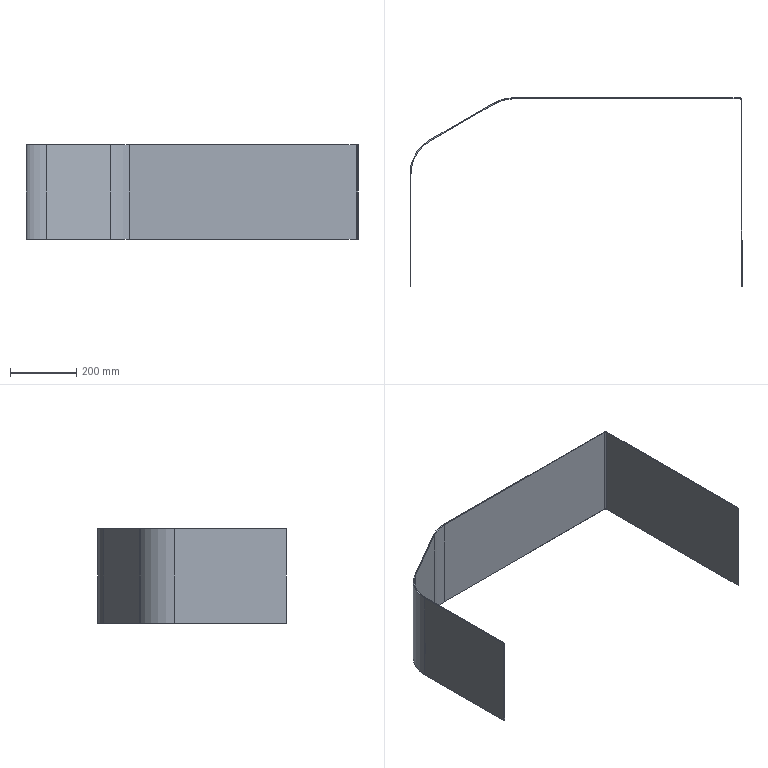Part | SolidWorks | features FlatPattern 1, SMBaseFlange 1, SheetMetal 1 | 1 solid | 30 faces | box 1004 x 570 x 285 mm | volume 1713041 mm3 | plane 24 | cylinder 6 | commonest cylinder face diameters 234 x2 240 x2 6 x1 12 x1
STEP:
#1=CARTESIAN_POINT('',(60.,442.117,285.));
#2=VERTEX_POINT('',#1);
#3=CARTESIAN_POINT('',(61.5,439.519,285.));
#4=VERTEX_POINT('',#3);
#5=CARTESIAN_POINT('',(60.,442.117,285.));
#6=DIRECTION('',(0.5,-0.866,0.));
#7=VECTOR('',#6,1000.);
#8=LINE('',#5,#7);
#9=EDGE_CURVE('',#2,#4,#8,.T.);
#10=ORIENTED_EDGE('',*,*,#9,.F.);
#11=CARTESIAN_POINT('',(0.,338.194,285.));
#12=VERTEX_POINT('',#11);
#13=CARTESIAN_POINT('',(120.,338.194,285.));
#14=DIRECTION('',(0.,0.,-1.));
#15=DIRECTION('',(-1.,0.,0.));
#16=AXIS2_PLACEMENT_3D('',#13,#14,#15);
#17=CIRCLE('',#16,120.);
#18=EDGE_CURVE('',#12,#2,#17,.T.);
#19=ORIENTED_EDGE('',*,*,#18,.F.);
#20=CARTESIAN_POINT('',(3.,338.194,285.));
#21=VERTEX_POINT('',#20);
#22=CARTESIAN_POINT('',(3.,338.194,285.));
#23=DIRECTION('',(-1.,0.,0.));
#24=VECTOR('',#23,1000.);
#25=LINE('',#22,#24);
#26=EDGE_CURVE('',#21,#12,#25,.T.);
#27=ORIENTED_EDGE('',*,*,#26,.F.);
#28=CARTESIAN_POINT('',(120.,338.194,285.));
#29=DIRECTION('',(0.,0.,-1.));
#30=DIRECTION('',(1.,0.,0.));
#31=AXIS2_PLACEMENT_3D('',#28,#29,#30);
#32=CIRCLE('',#31,117.);
#33=EDGE_CURVE('',#21,#4,#32,.T.);
#34=ORIENTED_EDGE('',*,*,#33,.T.);
#35=EDGE_LOOP('',(#10,#19,#27,#34));
#36=FACE_OUTER_BOUND('',#35,.T.);
#37=CARTESIAN_POINT('',(60.,442.117,285.));
#38=DIRECTION('',(0.,0.,1.));
#39=DIRECTION('',(1.,0.,0.));
#40=AXIS2_PLACEMENT_3D('',#37,#38,#39);
#41=PLANE('',#40);
#42=ADVANCED_FACE('',(#36),#41,.T.);
#43=CARTESIAN_POINT('',(252.958,553.521,285.));
#44=VERTEX_POINT('',#43);
#45=CARTESIAN_POINT('',(252.958,553.521,285.));
#46=DIRECTION('',(0.866,0.5,0.));
#47=VECTOR('',#46,1000.);
#48=LINE('',#45,#47);
#49=EDGE_CURVE('',#2,#44,#48,.T.);
#50=ORIENTED_EDGE('',*,*,#49,.F.);
#51=ORIENTED_EDGE('',*,*,#9,.T.);
#52=CARTESIAN_POINT('',(254.458,550.923,285.));
#53=VERTEX_POINT('',#52);
#54=CARTESIAN_POINT('',(254.458,550.923,285.));
#55=DIRECTION('',(0.866,0.5,0.));
#56=VECTOR('',#55,1000.);
#57=LINE('',#54,#56);
#58=EDGE_CURVE('',#4,#53,#57,.T.);
#59=ORIENTED_EDGE('',*,*,#58,.T.);
#60=CARTESIAN_POINT('',(254.458,550.923,285.));
#61=DIRECTION('',(-0.5,0.866,0.));
#62=VECTOR('',#61,1000.);
#63=LINE('',#60,#62);
#64=EDGE_CURVE('',#53,#44,#63,.T.);
#65=ORIENTED_EDGE('',*,*,#64,.T.);
#66=EDGE_LOOP('',(#50,#51,#59,#65));
#67=FACE_OUTER_BOUND('',#66,.T.);
#68=CARTESIAN_POINT('',(3.,338.194,285.));
#69=DIRECTION('',(0.,0.,1.));
#70=DIRECTION('',(1.,0.,0.));
#71=AXIS2_PLACEMENT_3D('',#68,#69,#70);
#72=PLANE('',#71);
#73=ADVANCED_FACE('',(#67),#72,.T.);
#74=CARTESIAN_POINT('',(0.,338.194,0.));
#75=VERTEX_POINT('',#74);
#76=CARTESIAN_POINT('',(3.,338.194,0.));
#77=VERTEX_POINT('',#76);
#78=CARTESIAN_POINT('',(0.,338.194,0.));
#79=DIRECTION('',(1.,0.,0.));
#80=VECTOR('',#79,1000.);
#81=LINE('',#78,#80);
#82=EDGE_CURVE('',#75,#77,#81,.T.);
#83=ORIENTED_EDGE('',*,*,#82,.F.);
#84=CARTESIAN_POINT('',(60.,442.117,0.));
#85=VERTEX_POINT('',#84);
#86=CARTESIAN_POINT('',(120.,338.194,0.));
#87=DIRECTION('',(0.,0.,-1.));
#88=DIRECTION('',(-1.,0.,0.));
#89=AXIS2_PLACEMENT_3D('',#86,#87,#88);
#90=CIRCLE('',#89,120.);
#91=EDGE_CURVE('',#75,#85,#90,.T.);
#92=ORIENTED_EDGE('',*,*,#91,.T.);
#93=CARTESIAN_POINT('',(61.5,439.519,0.));
#94=VERTEX_POINT('',#93);
#95=CARTESIAN_POINT('',(61.5,439.519,0.));
#96=DIRECTION('',(-0.5,0.866,0.));
#97=VECTOR('',#96,1000.);
#98=LINE('',#95,#97);
#99=EDGE_CURVE('',#94,#85,#98,.T.);
#100=ORIENTED_EDGE('',*,*,#99,.F.);
#101=CARTESIAN_POINT('',(120.,338.194,0.));
#102=DIRECTION('',(0.,0.,-1.));
#103=DIRECTION('',(1.,0.,0.));
#104=AXIS2_PLACEMENT_3D('',#101,#102,#103);
#105=CIRCLE('',#104,117.);
#106=EDGE_CURVE('',#77,#94,#105,.T.);
#107=ORIENTED_EDGE('',*,*,#106,.F.);
#108=EDGE_LOOP('',(#83,#92,#100,#107));
#109=FACE_OUTER_BOUND('',#108,.T.);
#110=CARTESIAN_POINT('',(0.,338.194,0.));
#111=DIRECTION('',(0.,0.,-1.));
#112=DIRECTION('',(-1.,0.,0.));
#113=AXIS2_PLACEMENT_3D('',#110,#111,#112);
#114=PLANE('',#113);
#115=ADVANCED_FACE('',(#109),#114,.T.);
#116=CARTESIAN_POINT('',(0.,0.,0.));
#117=VERTEX_POINT('',#116);
#118=CARTESIAN_POINT('',(0.,0.,0.));
#119=DIRECTION('',(0.,1.,0.));
#120=VECTOR('',#119,1000.);
#121=LINE('',#118,#120);
#122=EDGE_CURVE('',#117,#75,#121,.T.);
#123=ORIENTED_EDGE('',*,*,#122,.T.);
#124=ORIENTED_EDGE('',*,*,#82,.T.);
#125=CARTESIAN_POINT('',(3.,0.,0.));
#126=VERTEX_POINT('',#125);
#127=CARTESIAN_POINT('',(3.,0.,0.));
#128=DIRECTION('',(0.,1.,0.));
#129=VECTOR('',#128,1000.);
#130=LINE('',#127,#129);
#131=EDGE_CURVE('',#126,#77,#130,.T.);
#132=ORIENTED_EDGE('',*,*,#131,.F.);
#133=CARTESIAN_POINT('',(3.,0.,0.));
#134=DIRECTION('',(-1.,0.,0.));
#135=VECTOR('',#134,1000.);
#136=LINE('',#133,#135);
#137=EDGE_CURVE('',#126,#117,#136,.T.);
#138=ORIENTED_EDGE('',*,*,#137,.T.);
#139=EDGE_LOOP('',(#123,#124,#132,#138));
#140=FACE_OUTER_BOUND('',#139,.T.);
#141=CARTESIAN_POINT('',(61.5,439.519,0.));
#142=DIRECTION('',(0.,0.,-1.));
#143=DIRECTION('',(-1.,0.,0.));
#144=AXIS2_PLACEMENT_3D('',#141,#142,#143);
#145=PLANE('',#144);
#146=ADVANCED_FACE('',(#140),#145,.T.);
#147=CARTESIAN_POINT('',(312.958,569.598,285.));
#148=VERTEX_POINT('',#147);
#149=CARTESIAN_POINT('',(312.958,566.598,285.));
#150=VERTEX_POINT('',#149);
#151=CARTESIAN_POINT('',(312.958,569.598,285.));
#152=DIRECTION('',(0.,-1.,0.));
#153=VECTOR('',#152,1000.);
#154=LINE('',#151,#153);
#155=EDGE_CURVE('',#148,#150,#154,.T.);
#156=ORIENTED_EDGE('',*,*,#155,.F.);
#157=CARTESIAN_POINT('',(312.958,449.598,285.));
#158=DIRECTION('',(0.,0.,-1.));
#159=DIRECTION('',(-1.,0.,0.));
#160=AXIS2_PLACEMENT_3D('',#157,#158,#159);
#161=CIRCLE('',#160,120.);
#162=EDGE_CURVE('',#44,#148,#161,.T.);
#163=ORIENTED_EDGE('',*,*,#162,.F.);
#164=ORIENTED_EDGE('',*,*,#64,.F.);
#165=CARTESIAN_POINT('',(312.958,449.598,285.));
#166=DIRECTION('',(0.,0.,-1.));
#167=DIRECTION('',(1.,0.,0.));
#168=AXIS2_PLACEMENT_3D('',#165,#166,#167);
#169=CIRCLE('',#168,117.);
#170=EDGE_CURVE('',#53,#150,#169,.T.);
#171=ORIENTED_EDGE('',*,*,#170,.T.);
#172=EDGE_LOOP('',(#156,#163,#164,#171));
#173=FACE_OUTER_BOUND('',#172,.T.);
#174=CARTESIAN_POINT('',(312.958,569.598,285.));
#175=DIRECTION('',(0.,0.,1.));
#176=DIRECTION('',(1.,0.,0.));
#177=AXIS2_PLACEMENT_3D('',#174,#175,#176);
#178=PLANE('',#177);
#179=ADVANCED_FACE('',(#173),#178,.T.);
#180=CARTESIAN_POINT('',(998.304,569.598,285.));
#181=VERTEX_POINT('',#180);
#182=CARTESIAN_POINT('',(998.304,569.598,285.));
#183=DIRECTION('',(1.,0.,0.));
#184=VECTOR('',#183,1000.);
#185=LINE('',#182,#184);
#186=EDGE_CURVE('',#148,#181,#185,.T.);
#187=ORIENTED_EDGE('',*,*,#186,.F.);
#188=ORIENTED_EDGE('',*,*,#155,.T.);
#189=CARTESIAN_POINT('',(998.304,566.598,285.));
#190=VERTEX_POINT('',#189);
#191=CARTESIAN_POINT('',(998.304,566.598,285.));
#192=DIRECTION('',(1.,0.,0.));
#193=VECTOR('',#192,1000.);
#194=LINE('',#191,#193);
#195=EDGE_CURVE('',#150,#190,#194,.T.);
#196=ORIENTED_EDGE('',*,*,#195,.T.);
#197=CARTESIAN_POINT('',(998.304,566.598,285.));
#198=DIRECTION('',(0.,1.,0.));
#199=VECTOR('',#198,1000.);
#200=LINE('',#197,#199);
#201=EDGE_CURVE('',#190,#181,#200,.T.);
#202=ORIENTED_EDGE('',*,*,#201,.T.);
#203=EDGE_LOOP('',(#187,#188,#196,#202));
#204=FACE_OUTER_BOUND('',#203,.T.);
#205=CARTESIAN_POINT('',(254.458,550.923,285.));
#206=DIRECTION('',(0.,0.,1.));
#207=DIRECTION('',(1.,0.,0.));
#208=AXIS2_PLACEMENT_3D('',#205,#206,#207);
#209=PLANE('',#208);
#210=ADVANCED_FACE('',(#204),#209,.T.);
#211=CARTESIAN_POINT('',(252.958,553.521,0.));
#212=VERTEX_POINT('',#211);
#213=CARTESIAN_POINT('',(254.458,550.923,0.));
#214=VERTEX_POINT('',#213);
#215=CARTESIAN_POINT('',(252.958,553.521,0.));
#216=DIRECTION('',(0.5,-0.866,0.));
#217=VECTOR('',#216,1000.);
#218=LINE('',#215,#217);
#219=EDGE_CURVE('',#212,#214,#218,.T.);
#220=ORIENTED_EDGE('',*,*,#219,.F.);
#221=CARTESIAN_POINT('',(312.958,569.598,0.));
#222=VERTEX_POINT('',#221);
#223=CARTESIAN_POINT('',(312.958,449.598,0.));
#224=DIRECTION('',(0.,0.,-1.));
#225=DIRECTION('',(-1.,0.,0.));
#226=AXIS2_PLACEMENT_3D('',#223,#224,#225);
#227=CIRCLE('',#226,120.);
#228=EDGE_CURVE('',#212,#222,#227,.T.);
#229=ORIENTED_EDGE('',*,*,#228,.T.);
#230=CARTESIAN_POINT('',(312.958,566.598,0.));
#231=VERTEX_POINT('',#230);
#232=CARTESIAN_POINT('',(312.958,566.598,0.));
#233=DIRECTION('',(0.,1.,0.));
#234=VECTOR('',#233,1000.);
#235=LINE('',#232,#234);
#236=EDGE_CURVE('',#231,#222,#235,.T.);
#237=ORIENTED_EDGE('',*,*,#236,.F.);
#238=CARTESIAN_POINT('',(312.958,449.598,0.));
#239=DIRECTION('',(0.,0.,-1.));
#240=DIRECTION('',(1.,0.,0.));
#241=AXIS2_PLACEMENT_3D('',#238,#239,#240);
#242=CIRCLE('',#241,117.);
#243=EDGE_CURVE('',#214,#231,#242,.T.);
#244=ORIENTED_EDGE('',*,*,#243,.F.);
#245=EDGE_LOOP('',(#220,#229,#237,#244));
#246=FACE_OUTER_BOUND('',#245,.T.);
#247=CARTESIAN_POINT('',(252.958,553.521,0.));
#248=DIRECTION('',(0.,0.,-1.));
#249=DIRECTION('',(-1.,0.,0.));
#250=AXIS2_PLACEMENT_3D('',#247,#248,#249);
#251=PLANE('',#250);
#252=ADVANCED_FACE('',(#246),#251,.T.);
#253=CARTESIAN_POINT('',(252.958,553.521,0.));
#254=DIRECTION('',(0.866,0.5,0.));
#255=VECTOR('',#254,1000.);
#256=LINE('',#253,#255);
#257=EDGE_CURVE('',#85,#212,#256,.T.);
#258=ORIENTED_EDGE('',*,*,#257,.T.);
#259=ORIENTED_EDGE('',*,*,#219,.T.);
#260=CARTESIAN_POINT('',(254.458,550.923,0.));
#261=DIRECTION('',(0.866,0.5,0.));
#262=VECTOR('',#261,1000.);
#263=LINE('',#260,#262);
#264=EDGE_CURVE('',#94,#214,#263,.T.);
#265=ORIENTED_EDGE('',*,*,#264,.F.);
#266=ORIENTED_EDGE('',*,*,#99,.T.);
#267=EDGE_LOOP('',(#258,#259,#265,#266));
#268=FACE_OUTER_BOUND('',#267,.T.);
#269=CARTESIAN_POINT('',(312.958,566.598,0.));
#270=DIRECTION('',(0.,0.,-1.));
#271=DIRECTION('',(-1.,0.,0.));
#272=AXIS2_PLACEMENT_3D('',#269,#270,#271);
#273=PLANE('',#272);
#274=ADVANCED_FACE('',(#268),#273,.T.);
#275=CARTESIAN_POINT('',(1004.304,563.598,285.));
#276=VERTEX_POINT('',#275);
#277=CARTESIAN_POINT('',(1001.304,563.598,285.));
#278=VERTEX_POINT('',#277);
#279=CARTESIAN_POINT('',(1004.304,563.598,285.));
#280=DIRECTION('',(-1.,0.,0.));
#281=VECTOR('',#280,1000.);
#282=LINE('',#279,#281);
#283=EDGE_CURVE('',#276,#278,#282,.T.);
#284=ORIENTED_EDGE('',*,*,#283,.F.);
#285=CARTESIAN_POINT('',(998.304,563.598,285.));
#286=DIRECTION('',(0.,0.,-1.));
#287=DIRECTION('',(1.,0.,0.));
#288=AXIS2_PLACEMENT_3D('',#285,#286,#287);
#289=CIRCLE('',#288,6.);
#290=EDGE_CURVE('',#181,#276,#289,.T.);
#291=ORIENTED_EDGE('',*,*,#290,.F.);
#292=ORIENTED_EDGE('',*,*,#201,.F.);
#293=CARTESIAN_POINT('',(998.304,563.598,285.));
#294=DIRECTION('',(0.,0.,-1.));
#295=DIRECTION('',(1.,0.,0.));
#296=AXIS2_PLACEMENT_3D('',#293,#294,#295);
#297=CIRCLE('',#296,3.);
#298=EDGE_CURVE('',#190,#278,#297,.T.);
#299=ORIENTED_EDGE('',*,*,#298,.T.);
#300=EDGE_LOOP('',(#284,#291,#292,#299));
#301=FACE_OUTER_BOUND('',#300,.T.);
#302=CARTESIAN_POINT('',(1004.304,563.598,285.));
#303=DIRECTION('',(0.,0.,1.));
#304=DIRECTION('',(1.,0.,0.));
#305=AXIS2_PLACEMENT_3D('',#302,#303,#304);
#306=PLANE('',#305);
#307=ADVANCED_FACE('',(#301),#306,.T.);
#308=CARTESIAN_POINT('',(1004.304,-0.4019,285.));
#309=VERTEX_POINT('',#308);
#310=CARTESIAN_POINT('',(1004.304,563.598,285.));
#311=DIRECTION('',(0.,-1.,0.));
#312=VECTOR('',#311,1000.);
#313=LINE('',#310,#312);
#314=EDGE_CURVE('',#276,#309,#313,.T.);
#315=ORIENTED_EDGE('',*,*,#314,.F.);
#316=ORIENTED_EDGE('',*,*,#283,.T.);
#317=CARTESIAN_POINT('',(1001.304,-0.4019,285.));
#318=VERTEX_POINT('',#317);
#319=CARTESIAN_POINT('',(1001.304,563.598,285.));
#320=DIRECTION('',(0.,-1.,0.));
#321=VECTOR('',#320,1000.);
#322=LINE('',#319,#321);
#323=EDGE_CURVE('',#278,#318,#322,.T.);
#324=ORIENTED_EDGE('',*,*,#323,.T.);
#325=CARTESIAN_POINT('',(1004.304,-0.4019,285.));
#326=DIRECTION('',(-1.,0.,0.));
#327=VECTOR('',#326,1000.);
#328=LINE('',#325,#327);
#329=EDGE_CURVE('',#309,#318,#328,.T.);
#330=ORIENTED_EDGE('',*,*,#329,.F.);
#331=EDGE_LOOP('',(#315,#316,#324,#330));
#332=FACE_OUTER_BOUND('',#331,.T.);
#333=CARTESIAN_POINT('',(998.304,566.598,285.));
#334=DIRECTION('',(0.,0.,1.));
#335=DIRECTION('',(1.,0.,0.));
#336=AXIS2_PLACEMENT_3D('',#333,#334,#335);
#337=PLANE('',#336);
#338=ADVANCED_FACE('',(#332),#337,.T.);
#339=CARTESIAN_POINT('',(998.304,569.598,0.));
#340=VERTEX_POINT('',#339);
#341=CARTESIAN_POINT('',(998.304,566.598,0.));
#342=VERTEX_POINT('',#341);
#343=CARTESIAN_POINT('',(998.304,569.598,0.));
#344=DIRECTION('',(0.,-1.,0.));
#345=VECTOR('',#344,1000.);
#346=LINE('',#343,#345);
#347=EDGE_CURVE('',#340,#342,#346,.T.);
#348=ORIENTED_EDGE('',*,*,#347,.F.);
#349=CARTESIAN_POINT('',(1004.304,563.598,0.));
#350=VERTEX_POINT('',#349);
#351=CARTESIAN_POINT('',(998.304,563.598,0.));
#352=DIRECTION('',(0.,0.,-1.));
#353=DIRECTION('',(1.,0.,0.));
#354=AXIS2_PLACEMENT_3D('',#351,#352,#353);
#355=CIRCLE('',#354,6.);
#356=EDGE_CURVE('',#340,#350,#355,.T.);
#357=ORIENTED_EDGE('',*,*,#356,.T.);
#358=CARTESIAN_POINT('',(1001.304,563.598,0.));
#359=VERTEX_POINT('',#358);
#360=CARTESIAN_POINT('',(1001.304,563.598,0.));
#361=DIRECTION('',(1.,0.,0.));
#362=VECTOR('',#361,1000.);
#363=LINE('',#360,#362);
#364=EDGE_CURVE('',#359,#350,#363,.T.);
#365=ORIENTED_EDGE('',*,*,#364,.F.);
#366=CARTESIAN_POINT('',(998.304,563.598,0.));
#367=DIRECTION('',(0.,0.,-1.));
#368=DIRECTION('',(1.,0.,0.));
#369=AXIS2_PLACEMENT_3D('',#366,#367,#368);
#370=CIRCLE('',#369,3.);
#371=EDGE_CURVE('',#342,#359,#370,.T.);
#372=ORIENTED_EDGE('',*,*,#371,.F.);
#373=EDGE_LOOP('',(#348,#357,#365,#372));
#374=FACE_OUTER_BOUND('',#373,.T.);
#375=CARTESIAN_POINT('',(998.304,569.598,0.));
#376=DIRECTION('',(0.,0.,-1.));
#377=DIRECTION('',(-1.,0.,0.));
#378=AXIS2_PLACEMENT_3D('',#375,#376,#377);
#379=PLANE('',#378);
#380=ADVANCED_FACE('',(#374),#379,.T.);
#381=CARTESIAN_POINT('',(998.304,569.598,0.));
#382=DIRECTION('',(1.,0.,0.));
#383=VECTOR('',#382,1000.);
#384=LINE('',#381,#383);
#385=EDGE_CURVE('',#222,#340,#384,.T.);
#386=ORIENTED_EDGE('',*,*,#385,.T.);
#387=ORIENTED_EDGE('',*,*,#347,.T.);
#388=CARTESIAN_POINT('',(998.304,566.598,0.));
#389=DIRECTION('',(1.,0.,0.));
#390=VECTOR('',#389,1000.);
#391=LINE('',#388,#390);
#392=EDGE_CURVE('',#231,#342,#391,.T.);
#393=ORIENTED_EDGE('',*,*,#392,.F.);
#394=ORIENTED_EDGE('',*,*,#236,.T.);
#395=EDGE_LOOP('',(#386,#387,#393,#394));
#396=FACE_OUTER_BOUND('',#395,.T.);
#397=CARTESIAN_POINT('',(1001.304,563.598,0.));
#398=DIRECTION('',(0.,0.,-1.));
#399=DIRECTION('',(-1.,0.,0.));
#400=AXIS2_PLACEMENT_3D('',#397,#398,#399);
#401=PLANE('',#400);
#402=ADVANCED_FACE('',(#396),#401,.T.);
#403=CARTESIAN_POINT('',(1001.304,-0.4019,0.));
#404=VERTEX_POINT('',#403);
#405=CARTESIAN_POINT('',(1001.304,563.598,0.));
#406=DIRECTION('',(0.,-1.,0.));
#407=VECTOR('',#406,1000.);
#408=LINE('',#405,#407);
#409=EDGE_CURVE('',#359,#404,#408,.T.);
#410=ORIENTED_EDGE('',*,*,#409,.T.);
#411=CARTESIAN_POINT('',(1001.304,-0.4019,285.));
#412=DIRECTION('',(0.,0.,-1.));
#413=VECTOR('',#412,1000.);
#414=LINE('',#411,#413);
#415=EDGE_CURVE('',#318,#404,#414,.T.);
#416=ORIENTED_EDGE('',*,*,#415,.F.);
#417=ORIENTED_EDGE('',*,*,#323,.F.);
#418=CARTESIAN_POINT('',(1001.304,563.598,285.));
#419=DIRECTION('',(0.,0.,-1.));
#420=VECTOR('',#419,1000.);
#421=LINE('',#418,#420);
#422=EDGE_CURVE('',#278,#359,#421,.T.);
#423=ORIENTED_EDGE('',*,*,#422,.T.);
#424=EDGE_LOOP('',(#410,#416,#417,#423));
#425=FACE_OUTER_BOUND('',#424,.T.);
#426=CARTESIAN_POINT('',(1001.304,563.598,285.));
#427=DIRECTION('',(1.,0.,0.));
#428=DIRECTION('',(0.,1.,0.));
#429=AXIS2_PLACEMENT_3D('',#426,#427,#428);
#430=PLANE('',#429);
#431=ADVANCED_FACE('',(#425),#430,.F.);
#432=CARTESIAN_POINT('',(1004.304,-0.4019,0.));
#433=VERTEX_POINT('',#432);
#434=CARTESIAN_POINT('',(1004.304,-0.4019,0.));
#435=DIRECTION('',(-1.,0.,0.));
#436=VECTOR('',#435,1000.);
#437=LINE('',#434,#436);
#438=EDGE_CURVE('',#433,#404,#437,.T.);
#439=ORIENTED_EDGE('',*,*,#438,.F.);
#440=CARTESIAN_POINT('',(1004.304,-0.4019,285.));
#441=DIRECTION('',(0.,0.,-1.));
#442=VECTOR('',#441,1000.);
#443=LINE('',#440,#442);
#444=EDGE_CURVE('',#309,#433,#443,.T.);
#445=ORIENTED_EDGE('',*,*,#444,.F.);
#446=ORIENTED_EDGE('',*,*,#329,.T.);
#447=ORIENTED_EDGE('',*,*,#415,.T.);
#448=EDGE_LOOP('',(#439,#445,#446,#447));
#449=FACE_OUTER_BOUND('',#448,.T.);
#450=CARTESIAN_POINT('',(1004.304,-0.4019,285.));
#451=DIRECTION('',(0.,-1.,0.));
#452=DIRECTION('',(1.,0.,0.));
#453=AXIS2_PLACEMENT_3D('',#450,#451,#452);
#454=PLANE('',#453);
#455=ADVANCED_FACE('',(#449),#454,.T.);
#456=CARTESIAN_POINT('',(1004.304,563.598,0.));
#457=DIRECTION('',(0.,-1.,0.));
#458=VECTOR('',#457,1000.);
#459=LINE('',#456,#458);
#460=EDGE_CURVE('',#350,#433,#459,.T.);
#461=ORIENTED_EDGE('',*,*,#460,.F.);
#462=CARTESIAN_POINT('',(1004.304,563.598,285.));
#463=DIRECTION('',(0.,0.,-1.));
#464=VECTOR('',#463,1000.);
#465=LINE('',#462,#464);
#466=EDGE_CURVE('',#276,#350,#465,.T.);
#467=ORIENTED_EDGE('',*,*,#466,.F.);
#468=ORIENTED_EDGE('',*,*,#314,.T.);
#469=ORIENTED_EDGE('',*,*,#444,.T.);
#470=EDGE_LOOP('',(#461,#467,#468,#469));
#471=FACE_OUTER_BOUND('',#470,.T.);
#472=CARTESIAN_POINT('',(1004.304,563.598,285.));
#473=DIRECTION('',(1.,0.,0.));
#474=DIRECTION('',(0.,1.,0.));
#475=AXIS2_PLACEMENT_3D('',#472,#473,#474);
#476=PLANE('',#475);
#477=ADVANCED_FACE('',(#471),#476,.T.);
#478=ORIENTED_EDGE('',*,*,#356,.F.);
#479=CARTESIAN_POINT('',(998.304,569.598,285.));
#480=DIRECTION('',(0.,0.,-1.));
#481=VECTOR('',#480,1000.);
#482=LINE('',#479,#481);
#483=EDGE_CURVE('',#181,#340,#482,.T.);
#484=ORIENTED_EDGE('',*,*,#483,.F.);
#485=ORIENTED_EDGE('',*,*,#290,.T.);
#486=ORIENTED_EDGE('',*,*,#466,.T.);
#487=EDGE_LOOP('',(#478,#484,#485,#486));
#488=FACE_OUTER_BOUND('',#487,.T.);
#489=CARTESIAN_POINT('',(998.304,563.598,285.));
#490=DIRECTION('',(0.,0.,-1.));
#491=DIRECTION('',(-1.,0.,0.));
#492=AXIS2_PLACEMENT_3D('',#489,#490,#491);
#493=CYLINDRICAL_SURFACE('',#492,6.);
#494=ADVANCED_FACE('',(#488),#493,.T.);
#495=ORIENTED_EDGE('',*,*,#385,.F.);
#496=CARTESIAN_POINT('',(312.958,569.598,285.));
#497=DIRECTION('',(0.,0.,-1.));
#498=VECTOR('',#497,1000.);
#499=LINE('',#496,#498);
#500=EDGE_CURVE('',#148,#222,#499,.T.);
#501=ORIENTED_EDGE('',*,*,#500,.F.);
#502=ORIENTED_EDGE('',*,*,#186,.T.);
#503=ORIENTED_EDGE('',*,*,#483,.T.);
#504=EDGE_LOOP('',(#495,#501,#502,#503));
#505=FACE_OUTER_BOUND('',#504,.T.);
#506=CARTESIAN_POINT('',(998.304,569.598,285.));
#507=DIRECTION('',(0.,1.,0.));
#508=DIRECTION('',(0.,0.,1.));
#509=AXIS2_PLACEMENT_3D('',#506,#507,#508);
#510=PLANE('',#509);
#511=ADVANCED_FACE('',(#505),#510,.T.);
#512=ORIENTED_EDGE('',*,*,#228,.F.);
#513=CARTESIAN_POINT('',(252.958,553.521,285.));
#514=DIRECTION('',(0.,0.,-1.));
#515=VECTOR('',#514,1000.);
#516=LINE('',#513,#515);
#517=EDGE_CURVE('',#44,#212,#516,.T.);
#518=ORIENTED_EDGE('',*,*,#517,.F.);
#519=ORIENTED_EDGE('',*,*,#162,.T.);
#520=ORIENTED_EDGE('',*,*,#500,.T.);
#521=EDGE_LOOP('',(#512,#518,#519,#520));
#522=FACE_OUTER_BOUND('',#521,.T.);
#523=CARTESIAN_POINT('',(312.958,449.598,285.));
#524=DIRECTION('',(0.,0.,-1.));
#525=DIRECTION('',(-1.,0.,0.));
#526=AXIS2_PLACEMENT_3D('',#523,#524,#525);
#527=CYLINDRICAL_SURFACE('',#526,120.);
#528=ADVANCED_FACE('',(#522),#527,.T.);
#529=ORIENTED_EDGE('',*,*,#257,.F.);
#530=CARTESIAN_POINT('',(60.,442.117,285.));
#531=DIRECTION('',(0.,0.,-1.));
#532=VECTOR('',#531,1000.);
#533=LINE('',#530,#532);
#534=EDGE_CURVE('',#2,#85,#533,.T.);
#535=ORIENTED_EDGE('',*,*,#534,.F.);
#536=ORIENTED_EDGE('',*,*,#49,.T.);
#537=ORIENTED_EDGE('',*,*,#517,.T.);
#538=EDGE_LOOP('',(#529,#535,#536,#537));
#539=FACE_OUTER_BOUND('',#538,.T.);
#540=CARTESIAN_POINT('',(252.958,553.521,285.));
#541=DIRECTION('',(-0.5,0.866,0.));
#542=DIRECTION('',(-0.866,-0.5,0.));
#543=AXIS2_PLACEMENT_3D('',#540,#541,#542);
#544=PLANE('',#543);
#545=ADVANCED_FACE('',(#539),#544,.T.);
#546=ORIENTED_EDGE('',*,*,#91,.F.);
#547=CARTESIAN_POINT('',(0.,338.194,285.));
#548=DIRECTION('',(0.,0.,-1.));
#549=VECTOR('',#548,1000.);
#550=LINE('',#547,#549);
#551=EDGE_CURVE('',#12,#75,#550,.T.);
#552=ORIENTED_EDGE('',*,*,#551,.F.);
#553=ORIENTED_EDGE('',*,*,#18,.T.);
#554=ORIENTED_EDGE('',*,*,#534,.T.);
#555=EDGE_LOOP('',(#546,#552,#553,#554));
#556=FACE_OUTER_BOUND('',#555,.T.);
#557=CARTESIAN_POINT('',(120.,338.194,285.));
#558=DIRECTION('',(0.,0.,-1.));
#559=DIRECTION('',(-1.,0.,0.));
#560=AXIS2_PLACEMENT_3D('',#557,#558,#559);
#561=CYLINDRICAL_SURFACE('',#560,120.);
#562=ADVANCED_FACE('',(#556),#561,.T.);
#563=ORIENTED_EDGE('',*,*,#122,.F.);
#564=CARTESIAN_POINT('',(0.,0.,285.));
#565=VERTEX_POINT('',#564);
#566=CARTESIAN_POINT('',(0.,0.,285.));
#567=DIRECTION('',(0.,0.,-1.));
#568=VECTOR('',#567,1000.);
#569=LINE('',#566,#568);
#570=EDGE_CURVE('',#565,#117,#569,.T.);
#571=ORIENTED_EDGE('',*,*,#570,.F.);
#572=CARTESIAN_POINT('',(0.,0.,285.));
#573=DIRECTION('',(0.,1.,0.));
#574=VECTOR('',#573,1000.);
#575=LINE('',#572,#574);
#576=EDGE_CURVE('',#565,#12,#575,.T.);
#577=ORIENTED_EDGE('',*,*,#576,.T.);
#578=ORIENTED_EDGE('',*,*,#551,.T.);
#579=EDGE_LOOP('',(#563,#571,#577,#578));
#580=FACE_OUTER_BOUND('',#579,.T.);
#581=CARTESIAN_POINT('',(0.,0.,285.));
#582=DIRECTION('',(-1.,0.,0.));
#583=DIRECTION('',(0.,-1.,0.));
#584=AXIS2_PLACEMENT_3D('',#581,#582,#583);
#585=PLANE('',#584);
#586=ADVANCED_FACE('',(#580),#585,.T.);
#587=ORIENTED_EDGE('',*,*,#137,.F.);
#588=CARTESIAN_POINT('',(3.,0.,285.));
#589=VERTEX_POINT('',#588);
#590=CARTESIAN_POINT('',(3.,0.,285.));
#591=DIRECTION('',(0.,0.,-1.));
#592=VECTOR('',#591,1000.);
#593=LINE('',#590,#592);
#594=EDGE_CURVE('',#589,#126,#593,.T.);
#595=ORIENTED_EDGE('',*,*,#594,.F.);
#596=CARTESIAN_POINT('',(3.,0.,285.));
#597=DIRECTION('',(-1.,0.,0.));
#598=VECTOR('',#597,1000.);
#599=LINE('',#596,#598);
#600=EDGE_CURVE('',#589,#565,#599,.T.);
#601=ORIENTED_EDGE('',*,*,#600,.T.);
#602=ORIENTED_EDGE('',*,*,#570,.T.);
#603=EDGE_LOOP('',(#587,#595,#601,#602));
#604=FACE_OUTER_BOUND('',#603,.T.);
#605=CARTESIAN_POINT('',(3.,0.,285.));
#606=DIRECTION('',(0.,-1.,0.));
#607=DIRECTION('',(1.,0.,0.));
#608=AXIS2_PLACEMENT_3D('',#605,#606,#607);
#609=PLANE('',#608);
#610=ADVANCED_FACE('',(#604),#609,.T.);
#611=ORIENTED_EDGE('',*,*,#131,.T.);
#612=CARTESIAN_POINT('',(3.,338.194,285.));
#613=DIRECTION('',(0.,0.,-1.));
#614=VECTOR('',#613,1000.);
#615=LINE('',#612,#614);
#616=EDGE_CURVE('',#21,#77,#615,.T.);
#617=ORIENTED_EDGE('',*,*,#616,.F.);
#618=CARTESIAN_POINT('',(3.,0.,285.));
#619=DIRECTION('',(0.,1.,0.));
#620=VECTOR('',#619,1000.);
#621=LINE('',#618,#620);
#622=EDGE_CURVE('',#589,#21,#621,.T.);
#623=ORIENTED_EDGE('',*,*,#622,.F.);
#624=ORIENTED_EDGE('',*,*,#594,.T.);
#625=EDGE_LOOP('',(#611,#617,#623,#624));
#626=FACE_OUTER_BOUND('',#625,.T.);
#627=CARTESIAN_POINT('',(3.,0.,285.));
#628=DIRECTION('',(-1.,0.,0.));
#629=DIRECTION('',(0.,-1.,0.));
#630=AXIS2_PLACEMENT_3D('',#627,#628,#629);
#631=PLANE('',#630);
#632=ADVANCED_FACE('',(#626),#631,.F.);
#633=ORIENTED_EDGE('',*,*,#106,.T.);
#634=CARTESIAN_POINT('',(61.5,439.519,285.));
#635=DIRECTION('',(0.,0.,-1.));
#636=VECTOR('',#635,1000.);
#637=LINE('',#634,#636);
#638=EDGE_CURVE('',#4,#94,#637,.T.);
#639=ORIENTED_EDGE('',*,*,#638,.F.);
#640=ORIENTED_EDGE('',*,*,#33,.F.);
#641=ORIENTED_EDGE('',*,*,#616,.T.);
#642=EDGE_LOOP('',(#633,#639,#640,#641));
#643=FACE_OUTER_BOUND('',#642,.T.);
#644=CARTESIAN_POINT('',(120.,338.194,285.));
#645=DIRECTION('',(0.,0.,-1.));
#646=DIRECTION('',(-1.,0.,0.));
#647=AXIS2_PLACEMENT_3D('',#644,#645,#646);
#648=CYLINDRICAL_SURFACE('',#647,117.);
#649=ADVANCED_FACE('',(#643),#648,.F.);
#650=ORIENTED_EDGE('',*,*,#264,.T.);
#651=CARTESIAN_POINT('',(254.458,550.923,285.));
#652=DIRECTION('',(0.,0.,-1.));
#653=VECTOR('',#652,1000.);
#654=LINE('',#651,#653);
#655=EDGE_CURVE('',#53,#214,#654,.T.);
#656=ORIENTED_EDGE('',*,*,#655,.F.);
#657=ORIENTED_EDGE('',*,*,#58,.F.);
#658=ORIENTED_EDGE('',*,*,#638,.T.);
#659=EDGE_LOOP('',(#650,#656,#657,#658));
#660=FACE_OUTER_BOUND('',#659,.T.);
#661=CARTESIAN_POINT('',(254.458,550.923,285.));
#662=DIRECTION('',(-0.5,0.866,0.));
#663=DIRECTION('',(-0.866,-0.5,0.));
#664=AXIS2_PLACEMENT_3D('',#661,#662,#663);
#665=PLANE('',#664);
#666=ADVANCED_FACE('',(#660),#665,.F.);
#667=ORIENTED_EDGE('',*,*,#243,.T.);
#668=CARTESIAN_POINT('',(312.958,566.598,285.));
#669=DIRECTION('',(0.,0.,-1.));
#670=VECTOR('',#669,1000.);
#671=LINE('',#668,#670);
#672=EDGE_CURVE('',#150,#231,#671,.T.);
#673=ORIENTED_EDGE('',*,*,#672,.F.);
#674=ORIENTED_EDGE('',*,*,#170,.F.);
#675=ORIENTED_EDGE('',*,*,#655,.T.);
#676=EDGE_LOOP('',(#667,#673,#674,#675));
#677=FACE_OUTER_BOUND('',#676,.T.);
#678=CARTESIAN_POINT('',(312.958,449.598,285.));
#679=DIRECTION('',(0.,0.,-1.));
#680=DIRECTION('',(-1.,0.,0.));
#681=AXIS2_PLACEMENT_3D('',#678,#679,#680);
#682=CYLINDRICAL_SURFACE('',#681,117.);
#683=ADVANCED_FACE('',(#677),#682,.F.);
#684=ORIENTED_EDGE('',*,*,#392,.T.);
#685=CARTESIAN_POINT('',(998.304,566.598,285.));
#686=DIRECTION('',(0.,0.,-1.));
#687=VECTOR('',#686,1000.);
#688=LINE('',#685,#687);
#689=EDGE_CURVE('',#190,#342,#688,.T.);
#690=ORIENTED_EDGE('',*,*,#689,.F.);
#691=ORIENTED_EDGE('',*,*,#195,.F.);
#692=ORIENTED_EDGE('',*,*,#672,.T.);
#693=EDGE_LOOP('',(#684,#690,#691,#692));
#694=FACE_OUTER_BOUND('',#693,.T.);
#695=CARTESIAN_POINT('',(998.304,566.598,285.));
#696=DIRECTION('',(0.,1.,0.));
#697=DIRECTION('',(0.,0.,1.));
#698=AXIS2_PLACEMENT_3D('',#695,#696,#697);
#699=PLANE('',#698);
#700=ADVANCED_FACE('',(#694),#699,.F.);
#701=ORIENTED_EDGE('',*,*,#371,.T.);
#702=ORIENTED_EDGE('',*,*,#422,.F.);
#703=ORIENTED_EDGE('',*,*,#298,.F.);
#704=ORIENTED_EDGE('',*,*,#689,.T.);
#705=EDGE_LOOP('',(#701,#702,#703,#704));
#706=FACE_OUTER_BOUND('',#705,.T.);
#707=CARTESIAN_POINT('',(998.304,563.598,285.));
#708=DIRECTION('',(0.,0.,-1.));
#709=DIRECTION('',(-1.,0.,0.));
#710=AXIS2_PLACEMENT_3D('',#707,#708,#709);
#711=CYLINDRICAL_SURFACE('',#710,3.);
#712=ADVANCED_FACE('',(#706),#711,.F.);
#713=ORIENTED_EDGE('',*,*,#622,.T.);
#714=ORIENTED_EDGE('',*,*,#26,.T.);
#715=ORIENTED_EDGE('',*,*,#576,.F.);
#716=ORIENTED_EDGE('',*,*,#600,.F.);
#717=EDGE_LOOP('',(#713,#714,#715,#716));
#718=FACE_OUTER_BOUND('',#717,.T.);
#719=CARTESIAN_POINT('',(998.304,563.598,285.));
#720=DIRECTION('',(0.,0.,-1.));
#721=DIRECTION('',(-1.,0.,0.));
#722=AXIS2_PLACEMENT_3D('',#719,#720,#721);
#723=PLANE('',#722);
#724=ADVANCED_FACE('',(#718),#723,.F.);
#725=ORIENTED_EDGE('',*,*,#409,.F.);
#726=ORIENTED_EDGE('',*,*,#364,.T.);
#727=ORIENTED_EDGE('',*,*,#460,.T.);
#728=ORIENTED_EDGE('',*,*,#438,.T.);
#729=EDGE_LOOP('',(#725,#726,#727,#728));
#730=FACE_OUTER_BOUND('',#729,.T.);
#731=CARTESIAN_POINT('',(998.304,563.598,0.));
#732=DIRECTION('',(0.,0.,-1.));
#733=DIRECTION('',(-1.,0.,0.));
#734=AXIS2_PLACEMENT_3D('',#731,#732,#733);
#735=PLANE('',#734);
#736=ADVANCED_FACE('',(#730),#735,.T.);
#737=CLOSED_SHELL('',(#42,#73,#115,#146,#179,#210,#252,#274,#307,#338,#380,#402,#431,#455,#477,#494,#511,#528,#545,#562,#586,#610,#632,#649,#666,#683,#700,#712,#724,#736));
#738=MANIFOLD_SOLID_BREP('',#737);
#739=CARTESIAN_POINT('',(0.,0.,0.));
#740=DIRECTION('',(0.,0.,1.));
#741=DIRECTION('',(1.,0.,0.));
#742=AXIS2_PLACEMENT_3D('',#739,#740,#741);
#743=(LENGTH_UNIT()NAMED_UNIT(*)SI_UNIT(.MILLI.,.METRE.));
#744=UNCERTAINTY_MEASURE_WITH_UNIT(LENGTH_MEASURE(0.00001),#743,'','');
#745=(NAMED_UNIT(*)PLANE_ANGLE_UNIT()SI_UNIT($,.RADIAN.));
#746=(NAMED_UNIT(*)SI_UNIT($,.STERADIAN.)SOLID_ANGLE_UNIT());
#747=(GEOMETRIC_REPRESENTATION_CONTEXT(3)GLOBAL_UNCERTAINTY_ASSIGNED_CONTEXT((#744))GLOBAL_UNIT_ASSIGNED_CONTEXT((#743,#745,#746))REPRESENTATION_CONTEXT('',''));
#748=ADVANCED_BREP_SHAPE_REPRESENTATION('',(#738,#742),#747);